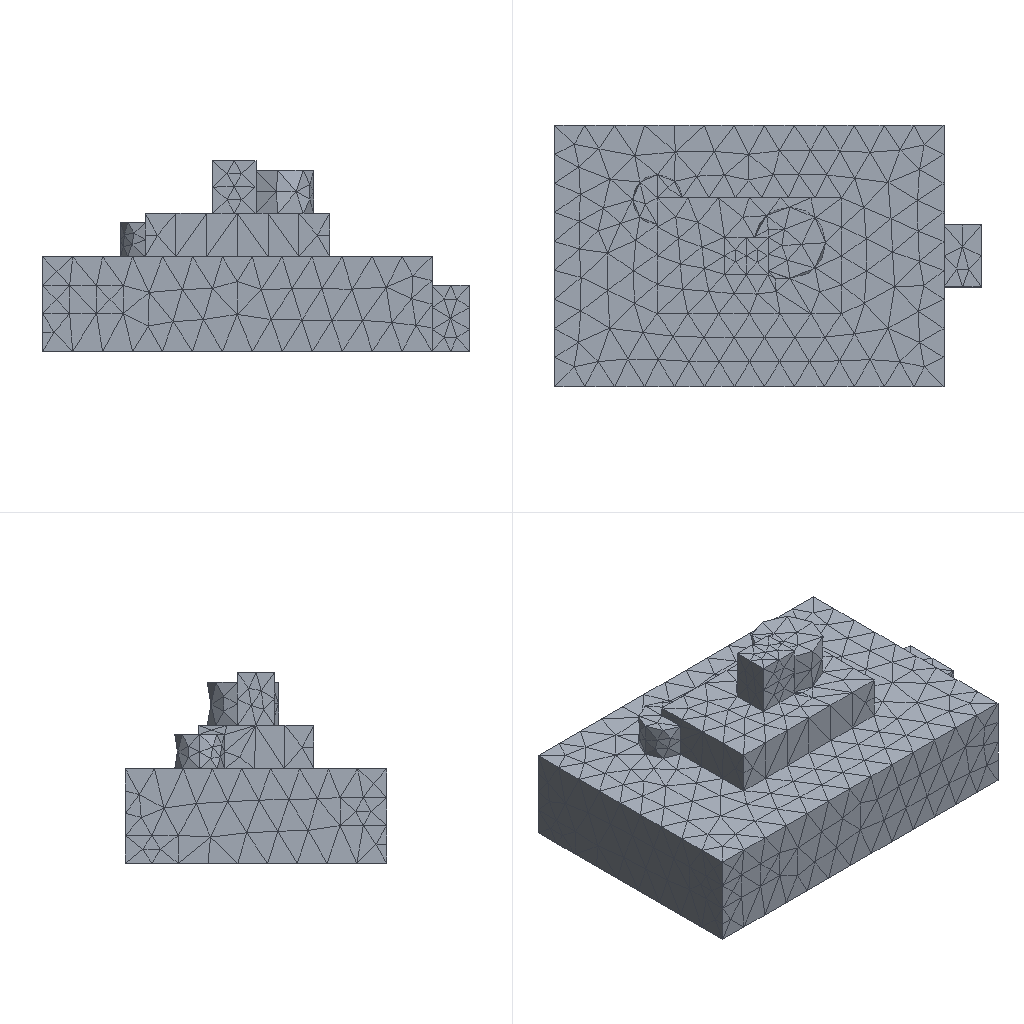Simulation study | ansys mapdl
Set-up summary:
category,name,step,type,value,unit,region
solver,ansys_mapdl
units,mm-N-s-tonne (MPa),,inferred,E=210000 density=
analysis,model,,static
mesh,nodes,,,6974
mesh,elements,,,4267
element_type,SOLID187,,,4267
material,mat 1,,E,210000
material,mat 1,,nu,0.3
load,,model,body load temp,,,all
load,,model,force,"1000 [dir=(0, 0, -1) n=386]",,node list
bc,,model,fixed,"[dofs=UX,UY,UZ n=7315]",,node list
Ansys APDL input file, long lists of numbers shortened:
/COM,ANSYS RELEASE 2026 R1           BUILD 26.1      UP20260202       09:08:11
/PREP7
/NOPR
/TITLE,2
ANTYPE, 0
*IF,_CDRDOFF,EQ,1,THEN     !if solid model was read in
_CDRDOFF=             !reset flag, numoffs already performed
*ELSE              !offset database for the following FE model
NUMOFF,NODE,     6974
NUMOFF,ELEM,     4267
NUMOFF,MAT ,        1
NUMOFF,TYPE,        1
*ENDIF
*SET,_RETURN ,  0.
*SET,_STATUS ,  0.
*SET,_UIQR   ,  386.
*SET,__FLOATPARAMETER__,  6974.
DOF,DELETE
ETBLOCK,        1,        1
(2i9,19a9)
        1      187        0        0        0        0        0        0        0        0        0        0        0        0        0        0        0        0        0        0        0
       -1
NBLOCK,6,SOLID,      6974,      6974
(3i9,6e21.13e3)
        1        0        0 6.0000000000000E+000 6.0000000000000E+000 6.1420000000000E+001
! (6973 more lines like these left out)
N,UNBL,LOC,       -1,
EBLOCK,19,SOLID,      4267,      4267
(19i10)
         1         1         1         1         0         0         0         0        10         0         1      2459      2460      2461      2462      2890      2891      2892      2893
! (8533 more lines like these left out)
        -1
MPTEMP,UNBL, 1, 1,  0.    ,
MPDATA,UNBL, 1,EX  ,       1, 1,  210000.000    ,
MPTEMP,UNBL, 1, 1,  0.    ,
MPDATA,UNBL, 1,NUXY,       1, 1, 0.3    ,
MPTEMP,UNBL, 1, 1,  0.    ,
MPDATA,UNBL, 1,PRXY,       1, 1, 0.3    ,
EXTOPT,ATTR,      0,      0,      0
EXTOPT,ESIZE,  0,  0.
EXTOPT,ACLEAR,      0
TREF,  0.
IRLF,  0
BFUNIF,TEMP,_TINY
ACEL,  0.    ,  0.    ,  0.
OMEGA,  0.    ,  0.    ,  0.
DOMEGA,  0.    ,  0.    ,  0.
CGLOC,  0.    ,  0.    ,  0.
CGOMEGA,  0.    ,  0.    ,  0.
DCGOMG,  0.    ,  0.    ,  0.
KUSE,     0
TIME,  0.
ALPHAD,  0.
BETAD,  0.
DMPRAT,  0.
DMPSTR,  0.
CRPLIM, 0.1    ,   0
CRPLIM,  0.    ,   1
NCNV,     0, 1.000000000E+12,     0,  0.    ,  0.
NEQIT,     0
ERESX,DEFA
DBLOCK,      7315
(i9,a6,2(pg16.9))
      566  UX    0.00000000      0.00000000
! (7314 more lines like these left out)
       -1
FBLOCK,       386
(i9,a6,2(pg16.9))
        1  FZ   -2.59067358      0.00000000
! (385 more lines like these left out)
       -1
/GO
FINISH
Results summary:
result,analysis_type_db,,,static,unstated
result,n_sets,,,1,unstated
result,load_steps[0].set,load_step=1,,1,unstated
result,load_steps[0].substep,load_step=1,,1,unstated
result,load_steps[0].time,load_step=1,,1,unstated
result,load_steps[0].freq,load_step=1,,1,unstated
result,load_steps[0].max_usum,load_step=1,,0.000395,unstated
result,load_steps[0].max_seqv,load_step=1,,3.539,unstated
result,load_steps[0].reaction_sum.FX,load_step=1,,-3.13536e-11,unstated
result,load_steps[0].reaction_sum.FY,load_step=1,,1.73287e-11,unstated
result,load_steps[0].reaction_sum.FZ,load_step=1,,1000,unstated
result,load_steps[0].reaction_sum.MX,load_step=1,,0,unstated
result,load_steps[0].reaction_sum.MY,load_step=1,,0,unstated
result,load_steps[0].reaction_sum.MZ,load_step=1,,0,unstated
result,convergence,,,results present for all listed sets,unstated